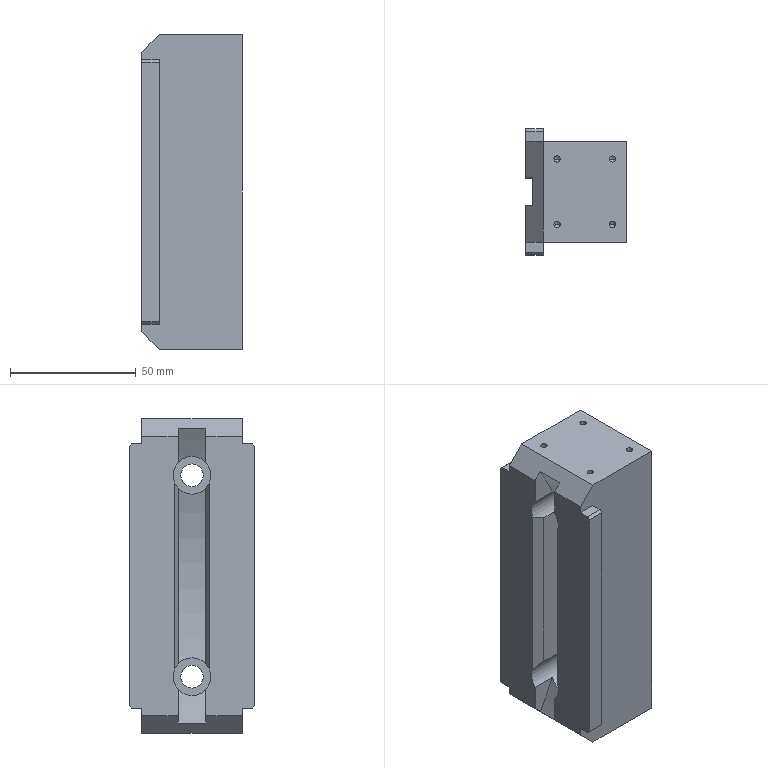Part | STEP file | Nylon Claw M20 | 1 solid | 58 faces | box 40 x 50 x 125 mm | volume 179842 mm3 | plane 31 | cylinder 19 | cone 8 | commonest cylinder face diameters 2.5 x8 9 x4 15 x4 228 x3